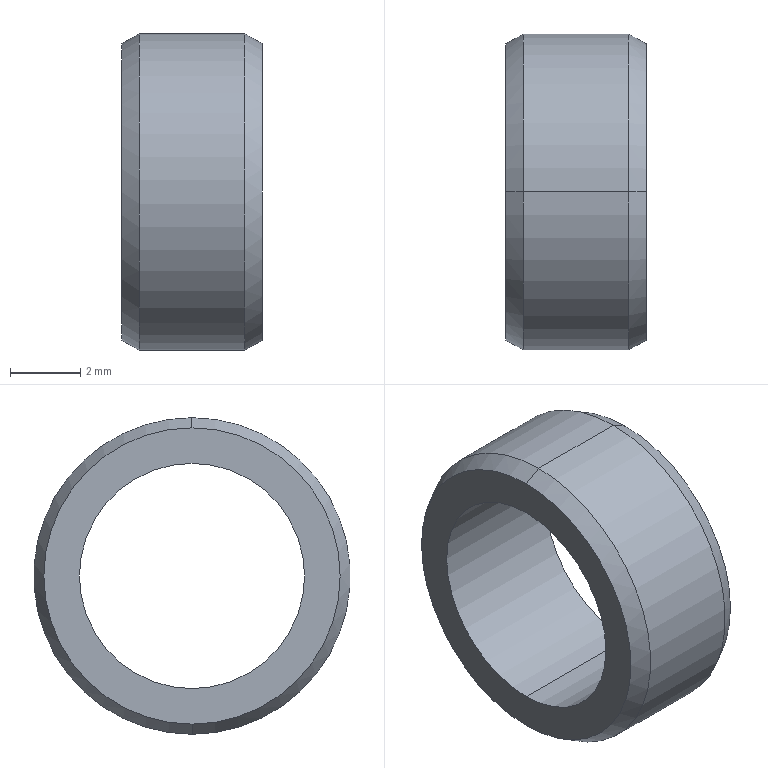Part | SolidWorks | features BaseBody 1 | 1 solid | 10 faces | box 4 x 9 x 9 mm | volume 121.796 mm3 | cylinder 4 | cone 4 | plane 2 | commonest cylinder face diameters 6.4 x2 9 x2
STEP:
#1=CARTESIAN_POINT('',(3.5,0.,4.5));
#2=VERTEX_POINT('',#1);
#3=CARTESIAN_POINT('',(3.5,0.,-4.5));
#4=VERTEX_POINT('',#3);
#5=CARTESIAN_POINT('',(3.5,0.,0.));
#6=DIRECTION('',(-1.,0.,0.));
#7=DIRECTION('',(0.,0.,1.));
#8=AXIS2_PLACEMENT_3D('',#5,#6,#7);
#9=CIRCLE('',#8,4.5);
#10=EDGE_CURVE('',#2,#4,#9,.T.);
#11=ORIENTED_EDGE('',*,*,#10,.T.);
#12=CARTESIAN_POINT('',(0.5,0.,-4.5));
#13=VERTEX_POINT('',#12);
#14=CARTESIAN_POINT('',(4.,0.,-4.5));
#15=DIRECTION('',(-1.,0.,0.));
#16=VECTOR('',#15,1000.);
#17=LINE('',#14,#16);
#18=EDGE_CURVE('',#4,#13,#17,.T.);
#19=ORIENTED_EDGE('',*,*,#18,.T.);
#20=CARTESIAN_POINT('',(0.5,0.,4.5));
#21=VERTEX_POINT('',#20);
#22=CARTESIAN_POINT('',(0.5,0.,0.));
#23=DIRECTION('',(1.,0.,0.));
#24=DIRECTION('',(0.,0.,1.));
#25=AXIS2_PLACEMENT_3D('',#22,#23,#24);
#26=CIRCLE('',#25,4.5);
#27=EDGE_CURVE('',#13,#21,#26,.T.);
#28=ORIENTED_EDGE('',*,*,#27,.T.);
#29=CARTESIAN_POINT('',(4.,0.,4.5));
#30=DIRECTION('',(-1.,0.,0.));
#31=VECTOR('',#30,1000.);
#32=LINE('',#29,#31);
#33=EDGE_CURVE('',#2,#21,#32,.T.);
#34=ORIENTED_EDGE('',*,*,#33,.F.);
#35=EDGE_LOOP('',(#11,#19,#28,#34));
#36=FACE_OUTER_BOUND('',#35,.T.);
#37=CARTESIAN_POINT('',(4.,0.,0.));
#38=DIRECTION('',(-1.,0.,0.));
#39=DIRECTION('',(0.,0.,1.));
#40=AXIS2_PLACEMENT_3D('',#37,#38,#39);
#41=CYLINDRICAL_SURFACE('',#40,4.5);
#42=ADVANCED_FACE('',(#36),#41,.T.);
#43=CARTESIAN_POINT('',(4.,0.,4.211));
#44=VERTEX_POINT('',#43);
#45=CARTESIAN_POINT('',(4.,0.,-4.211));
#46=VERTEX_POINT('',#45);
#47=CARTESIAN_POINT('',(4.,0.,0.));
#48=DIRECTION('',(-1.,0.,0.));
#49=DIRECTION('',(0.,0.,1.));
#50=AXIS2_PLACEMENT_3D('',#47,#48,#49);
#51=CIRCLE('',#50,4.211);
#52=EDGE_CURVE('',#44,#46,#51,.T.);
#53=ORIENTED_EDGE('',*,*,#52,.T.);
#54=CARTESIAN_POINT('',(3.5,0.,-4.5));
#55=DIRECTION('',(-0.866,0.,-0.5));
#56=VECTOR('',#55,1000.);
#57=LINE('',#54,#56);
#58=EDGE_CURVE('',#46,#4,#57,.T.);
#59=ORIENTED_EDGE('',*,*,#58,.T.);
#60=ORIENTED_EDGE('',*,*,#10,.F.);
#61=CARTESIAN_POINT('',(3.5,0.,4.5));
#62=DIRECTION('',(-0.866,0.,0.5));
#63=VECTOR('',#62,1000.);
#64=LINE('',#61,#63);
#65=EDGE_CURVE('',#44,#2,#64,.T.);
#66=ORIENTED_EDGE('',*,*,#65,.F.);
#67=EDGE_LOOP('',(#53,#59,#60,#66));
#68=FACE_OUTER_BOUND('',#67,.T.);
#69=CARTESIAN_POINT('',(3.5,0.,0.));
#70=DIRECTION('',(-1.,0.,0.));
#71=DIRECTION('',(0.,0.,1.));
#72=AXIS2_PLACEMENT_3D('',#69,#70,#71);
#73=CONICAL_SURFACE('',#72,4.5,0.5236);
#74=ADVANCED_FACE('',(#68),#73,.T.);
#75=CARTESIAN_POINT('',(0.,0.,-4.211));
#76=VERTEX_POINT('',#75);
#77=CARTESIAN_POINT('',(0.,0.,4.211));
#78=VERTEX_POINT('',#77);
#79=CARTESIAN_POINT('',(0.,0.,0.));
#80=DIRECTION('',(1.,0.,0.));
#81=DIRECTION('',(0.,0.,-1.));
#82=AXIS2_PLACEMENT_3D('',#79,#80,#81);
#83=CIRCLE('',#82,4.211);
#84=EDGE_CURVE('',#76,#78,#83,.T.);
#85=ORIENTED_EDGE('',*,*,#84,.T.);
#86=CARTESIAN_POINT('',(0.5,0.,4.5));
#87=DIRECTION('',(0.866,0.,0.5));
#88=VECTOR('',#87,1000.);
#89=LINE('',#86,#88);
#90=EDGE_CURVE('',#78,#21,#89,.T.);
#91=ORIENTED_EDGE('',*,*,#90,.T.);
#92=ORIENTED_EDGE('',*,*,#27,.F.);
#93=CARTESIAN_POINT('',(0.5,0.,-4.5));
#94=DIRECTION('',(0.866,0.,-0.5));
#95=VECTOR('',#94,1000.);
#96=LINE('',#93,#95);
#97=EDGE_CURVE('',#76,#13,#96,.T.);
#98=ORIENTED_EDGE('',*,*,#97,.F.);
#99=EDGE_LOOP('',(#85,#91,#92,#98));
#100=FACE_OUTER_BOUND('',#99,.T.);
#101=CARTESIAN_POINT('',(0.5,0.,0.));
#102=DIRECTION('',(1.,0.,0.));
#103=DIRECTION('',(0.,0.,-1.));
#104=AXIS2_PLACEMENT_3D('',#101,#102,#103);
#105=CONICAL_SURFACE('',#104,4.5,0.5236);
#106=ADVANCED_FACE('',(#100),#105,.T.);
#107=CARTESIAN_POINT('',(4.,0.,-3.2));
#108=VERTEX_POINT('',#107);
#109=CARTESIAN_POINT('',(4.,0.,3.2));
#110=VERTEX_POINT('',#109);
#111=CARTESIAN_POINT('',(4.,0.,0.));
#112=DIRECTION('',(-1.,0.,0.));
#113=DIRECTION('',(0.,0.,1.));
#114=AXIS2_PLACEMENT_3D('',#111,#112,#113);
#115=CIRCLE('',#114,3.2);
#116=EDGE_CURVE('',#108,#110,#115,.T.);
#117=ORIENTED_EDGE('',*,*,#116,.F.);
#118=CARTESIAN_POINT('',(0.,0.,-3.2));
#119=VERTEX_POINT('',#118);
#120=CARTESIAN_POINT('',(4.,0.,-3.2));
#121=DIRECTION('',(-1.,0.,0.));
#122=VECTOR('',#121,1000.);
#123=LINE('',#120,#122);
#124=EDGE_CURVE('',#108,#119,#123,.T.);
#125=ORIENTED_EDGE('',*,*,#124,.T.);
#126=CARTESIAN_POINT('',(0.,0.,3.2));
#127=VERTEX_POINT('',#126);
#128=CARTESIAN_POINT('',(0.,0.,0.));
#129=DIRECTION('',(1.,0.,0.));
#130=DIRECTION('',(0.,0.,1.));
#131=AXIS2_PLACEMENT_3D('',#128,#129,#130);
#132=CIRCLE('',#131,3.2);
#133=EDGE_CURVE('',#127,#119,#132,.T.);
#134=ORIENTED_EDGE('',*,*,#133,.F.);
#135=CARTESIAN_POINT('',(4.,0.,3.2));
#136=DIRECTION('',(-1.,0.,0.));
#137=VECTOR('',#136,1000.);
#138=LINE('',#135,#137);
#139=EDGE_CURVE('',#110,#127,#138,.T.);
#140=ORIENTED_EDGE('',*,*,#139,.F.);
#141=EDGE_LOOP('',(#117,#125,#134,#140));
#142=FACE_OUTER_BOUND('',#141,.T.);
#143=CARTESIAN_POINT('',(4.,0.,0.));
#144=DIRECTION('',(-1.,0.,0.));
#145=DIRECTION('',(0.,0.,1.));
#146=AXIS2_PLACEMENT_3D('',#143,#144,#145);
#147=CYLINDRICAL_SURFACE('',#146,3.2);
#148=ADVANCED_FACE('',(#142),#147,.F.);
#149=ORIENTED_EDGE('',*,*,#18,.F.);
#150=CARTESIAN_POINT('',(3.5,0.,0.));
#151=DIRECTION('',(-1.,0.,0.));
#152=DIRECTION('',(0.,0.,1.));
#153=AXIS2_PLACEMENT_3D('',#150,#151,#152);
#154=CIRCLE('',#153,4.5);
#155=EDGE_CURVE('',#4,#2,#154,.T.);
#156=ORIENTED_EDGE('',*,*,#155,.T.);
#157=ORIENTED_EDGE('',*,*,#33,.T.);
#158=CARTESIAN_POINT('',(0.5,0.,0.));
#159=DIRECTION('',(1.,0.,0.));
#160=DIRECTION('',(0.,0.,1.));
#161=AXIS2_PLACEMENT_3D('',#158,#159,#160);
#162=CIRCLE('',#161,4.5);
#163=EDGE_CURVE('',#21,#13,#162,.T.);
#164=ORIENTED_EDGE('',*,*,#163,.T.);
#165=EDGE_LOOP('',(#149,#156,#157,#164));
#166=FACE_OUTER_BOUND('',#165,.T.);
#167=CARTESIAN_POINT('',(4.,0.,0.));
#168=DIRECTION('',(-1.,0.,0.));
#169=DIRECTION('',(0.,0.,1.));
#170=AXIS2_PLACEMENT_3D('',#167,#168,#169);
#171=CYLINDRICAL_SURFACE('',#170,4.5);
#172=ADVANCED_FACE('',(#166),#171,.T.);
#173=ORIENTED_EDGE('',*,*,#58,.F.);
#174=CARTESIAN_POINT('',(4.,0.,0.));
#175=DIRECTION('',(-1.,0.,0.));
#176=DIRECTION('',(0.,0.,1.));
#177=AXIS2_PLACEMENT_3D('',#174,#175,#176);
#178=CIRCLE('',#177,4.211);
#179=EDGE_CURVE('',#46,#44,#178,.T.);
#180=ORIENTED_EDGE('',*,*,#179,.T.);
#181=ORIENTED_EDGE('',*,*,#65,.T.);
#182=ORIENTED_EDGE('',*,*,#155,.F.);
#183=EDGE_LOOP('',(#173,#180,#181,#182));
#184=FACE_OUTER_BOUND('',#183,.T.);
#185=CARTESIAN_POINT('',(3.5,0.,0.));
#186=DIRECTION('',(-1.,0.,0.));
#187=DIRECTION('',(0.,0.,1.));
#188=AXIS2_PLACEMENT_3D('',#185,#186,#187);
#189=CONICAL_SURFACE('',#188,4.5,0.5236);
#190=ADVANCED_FACE('',(#184),#189,.T.);
#191=ORIENTED_EDGE('',*,*,#90,.F.);
#192=CARTESIAN_POINT('',(0.,0.,0.));
#193=DIRECTION('',(1.,0.,0.));
#194=DIRECTION('',(0.,0.,-1.));
#195=AXIS2_PLACEMENT_3D('',#192,#193,#194);
#196=CIRCLE('',#195,4.211);
#197=EDGE_CURVE('',#78,#76,#196,.T.);
#198=ORIENTED_EDGE('',*,*,#197,.T.);
#199=ORIENTED_EDGE('',*,*,#97,.T.);
#200=ORIENTED_EDGE('',*,*,#163,.F.);
#201=EDGE_LOOP('',(#191,#198,#199,#200));
#202=FACE_OUTER_BOUND('',#201,.T.);
#203=CARTESIAN_POINT('',(0.5,0.,0.));
#204=DIRECTION('',(1.,0.,0.));
#205=DIRECTION('',(0.,0.,-1.));
#206=AXIS2_PLACEMENT_3D('',#203,#204,#205);
#207=CONICAL_SURFACE('',#206,4.5,0.5236);
#208=ADVANCED_FACE('',(#202),#207,.T.);
#209=CARTESIAN_POINT('',(4.,0.,0.));
#210=DIRECTION('',(-1.,0.,0.));
#211=DIRECTION('',(0.,0.,1.));
#212=AXIS2_PLACEMENT_3D('',#209,#210,#211);
#213=CIRCLE('',#212,3.2);
#214=EDGE_CURVE('',#110,#108,#213,.T.);
#215=ORIENTED_EDGE('',*,*,#214,.T.);
#216=ORIENTED_EDGE('',*,*,#116,.T.);
#217=EDGE_LOOP('',(#215,#216));
#218=FACE_BOUND('',#217,.T.);
#219=ORIENTED_EDGE('',*,*,#52,.F.);
#220=ORIENTED_EDGE('',*,*,#179,.F.);
#221=EDGE_LOOP('',(#219,#220));
#222=FACE_OUTER_BOUND('',#221,.T.);
#223=CARTESIAN_POINT('',(4.,3.2,0.));
#224=DIRECTION('',(1.,0.,0.));
#225=DIRECTION('',(0.,0.,-1.));
#226=AXIS2_PLACEMENT_3D('',#223,#224,#225);
#227=PLANE('',#226);
#228=ADVANCED_FACE('',(#218,#222),#227,.T.);
#229=ORIENTED_EDGE('',*,*,#84,.F.);
#230=ORIENTED_EDGE('',*,*,#197,.F.);
#231=EDGE_LOOP('',(#229,#230));
#232=FACE_OUTER_BOUND('',#231,.T.);
#233=ORIENTED_EDGE('',*,*,#133,.T.);
#234=CARTESIAN_POINT('',(0.,0.,0.));
#235=DIRECTION('',(1.,0.,0.));
#236=DIRECTION('',(0.,0.,1.));
#237=AXIS2_PLACEMENT_3D('',#234,#235,#236);
#238=CIRCLE('',#237,3.2);
#239=EDGE_CURVE('',#119,#127,#238,.T.);
#240=ORIENTED_EDGE('',*,*,#239,.T.);
#241=EDGE_LOOP('',(#233,#240));
#242=FACE_BOUND('',#241,.T.);
#243=CARTESIAN_POINT('',(0.,4.211,0.));
#244=DIRECTION('',(-1.,0.,0.));
#245=DIRECTION('',(0.,0.,1.));
#246=AXIS2_PLACEMENT_3D('',#243,#244,#245);
#247=PLANE('',#246);
#248=ADVANCED_FACE('',(#232,#242),#247,.T.);
#249=ORIENTED_EDGE('',*,*,#124,.F.);
#250=ORIENTED_EDGE('',*,*,#214,.F.);
#251=ORIENTED_EDGE('',*,*,#139,.T.);
#252=ORIENTED_EDGE('',*,*,#239,.F.);
#253=EDGE_LOOP('',(#249,#250,#251,#252));
#254=FACE_OUTER_BOUND('',#253,.T.);
#255=CARTESIAN_POINT('',(4.,0.,0.));
#256=DIRECTION('',(-1.,0.,0.));
#257=DIRECTION('',(0.,0.,1.));
#258=AXIS2_PLACEMENT_3D('',#255,#256,#257);
#259=CYLINDRICAL_SURFACE('',#258,3.2);
#260=ADVANCED_FACE('',(#254),#259,.F.);
#261=CLOSED_SHELL('',(#42,#74,#106,#148,#172,#190,#208,#228,#248,#260));
#262=MANIFOLD_SOLID_BREP('',#261);
#263=CARTESIAN_POINT('',(0.,0.,0.));
#264=DIRECTION('',(0.,0.,1.));
#265=DIRECTION('',(1.,0.,0.));
#266=AXIS2_PLACEMENT_3D('',#263,#264,#265);
#267=(LENGTH_UNIT()NAMED_UNIT(*)SI_UNIT(.MILLI.,.METRE.));
#268=UNCERTAINTY_MEASURE_WITH_UNIT(LENGTH_MEASURE(0.00001),#267,'','');
#269=(NAMED_UNIT(*)PLANE_ANGLE_UNIT()SI_UNIT($,.RADIAN.));
#270=(NAMED_UNIT(*)SI_UNIT($,.STERADIAN.)SOLID_ANGLE_UNIT());
#271=(GEOMETRIC_REPRESENTATION_CONTEXT(3)GLOBAL_UNCERTAINTY_ASSIGNED_CONTEXT((#268))GLOBAL_UNIT_ASSIGNED_CONTEXT((#267,#269,#270))REPRESENTATION_CONTEXT('',''));
#272=ADVANCED_BREP_SHAPE_REPRESENTATION('',(#262,#266),#271);